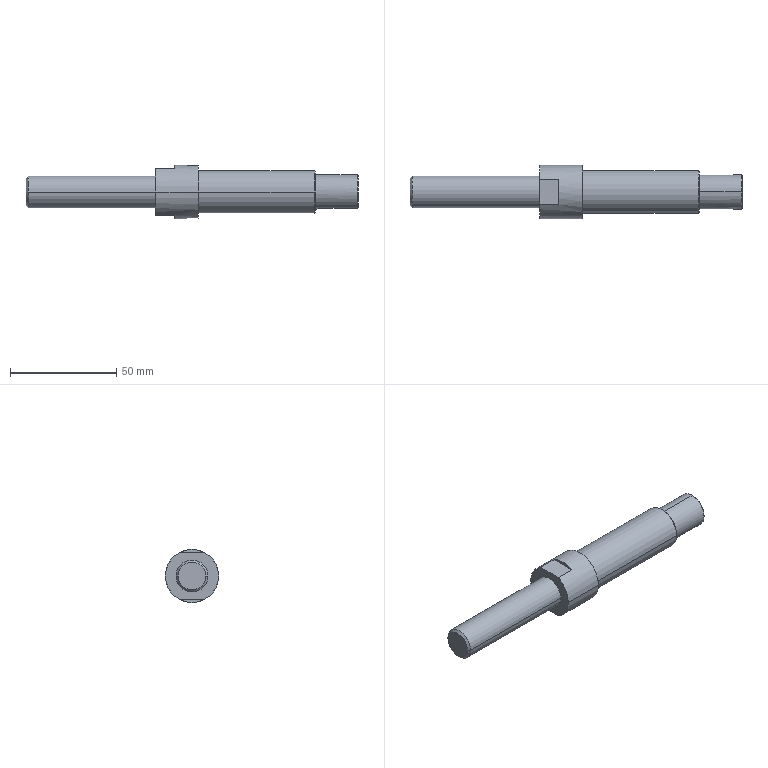Part | NX | 1 solid | 29 faces | box 156 x 25 x 25 mm | volume 41405 mm3 | plane 12 | cylinder 10 | cone 7 | commonest cylinder face diameters 5 x2 15 x2 16 x2 20 x2 25 x2
STEP:
#1=CARTESIAN_POINT('',(1862.,-10.,0.));
#2=VERTEX_POINT('',#1);
#3=CARTESIAN_POINT('',(1862.,10.,0.));
#4=VERTEX_POINT('',#3);
#5=CARTESIAN_POINT('',(1862.,0.,0.));
#6=DIRECTION('',(1.,0.,0.));
#7=DIRECTION('',(0.,1.,0.));
#8=AXIS2_PLACEMENT_3D('',#5,#6,#7);
#9=CIRCLE('',#8,10.);
#10=EDGE_CURVE('',#2,#4,#9,.T.);
#11=ORIENTED_EDGE('',*,*,#10,.T.);
#12=CARTESIAN_POINT('',(1916.5,10.,0.));
#13=VERTEX_POINT('',#12);
#14=CARTESIAN_POINT('',(1862.,10.,0.));
#15=DIRECTION('',(1.,0.,0.));
#16=VECTOR('',#15,1000.);
#17=LINE('',#14,#16);
#18=EDGE_CURVE('',#4,#13,#17,.T.);
#19=ORIENTED_EDGE('',*,*,#18,.T.);
#20=CARTESIAN_POINT('',(1916.5,-10.,0.));
#21=VERTEX_POINT('',#20);
#22=CARTESIAN_POINT('',(1916.5,0.,0.));
#23=DIRECTION('',(-1.,0.,0.));
#24=DIRECTION('',(0.,1.,0.));
#25=AXIS2_PLACEMENT_3D('',#22,#23,#24);
#26=CIRCLE('',#25,10.);
#27=EDGE_CURVE('',#13,#21,#26,.T.);
#28=ORIENTED_EDGE('',*,*,#27,.T.);
#29=CARTESIAN_POINT('',(1862.,-10.,0.));
#30=DIRECTION('',(1.,0.,0.));
#31=VECTOR('',#30,1000.);
#32=LINE('',#29,#31);
#33=EDGE_CURVE('',#2,#21,#32,.T.);
#34=ORIENTED_EDGE('',*,*,#33,.F.);
#35=EDGE_LOOP('',(#11,#19,#28,#34));
#36=FACE_BOUND('',#35,.T.);
#37=CARTESIAN_POINT('',(1862.,0.,0.));
#38=DIRECTION('',(1.,0.,0.));
#39=DIRECTION('',(0.,1.,0.));
#40=AXIS2_PLACEMENT_3D('',#37,#38,#39);
#41=CYLINDRICAL_SURFACE('',#40,10.);
#42=ADVANCED_FACE('',(#36),#41,.T.);
#43=CARTESIAN_POINT('',(1862.,12.5,0.));
#44=VERTEX_POINT('',#43);
#45=CARTESIAN_POINT('',(1862.,-12.5,0.));
#46=VERTEX_POINT('',#45);
#47=CARTESIAN_POINT('',(1862.,0.,0.));
#48=DIRECTION('',(-1.,0.,0.));
#49=DIRECTION('',(0.,1.,0.));
#50=AXIS2_PLACEMENT_3D('',#47,#48,#49);
#51=CIRCLE('',#50,12.5);
#52=EDGE_CURVE('',#44,#46,#51,.T.);
#53=ORIENTED_EDGE('',*,*,#52,.F.);
#54=CARTESIAN_POINT('',(1862.,0.,0.));
#55=DIRECTION('',(-1.,0.,0.));
#56=DIRECTION('',(0.,1.,0.));
#57=AXIS2_PLACEMENT_3D('',#54,#55,#56);
#58=CIRCLE('',#57,12.5);
#59=EDGE_CURVE('',#46,#44,#58,.T.);
#60=ORIENTED_EDGE('',*,*,#59,.F.);
#61=EDGE_LOOP('',(#53,#60));
#62=FACE_BOUND('',#61,.T.);
#63=ORIENTED_EDGE('',*,*,#10,.F.);
#64=CARTESIAN_POINT('',(1862.,0.,0.));
#65=DIRECTION('',(1.,0.,0.));
#66=DIRECTION('',(0.,1.,0.));
#67=AXIS2_PLACEMENT_3D('',#64,#65,#66);
#68=CIRCLE('',#67,10.);
#69=EDGE_CURVE('',#4,#2,#68,.T.);
#70=ORIENTED_EDGE('',*,*,#69,.F.);
#71=EDGE_LOOP('',(#63,#70));
#72=FACE_BOUND('',#71,.T.);
#73=CARTESIAN_POINT('',(1862.,-2.339,-2.068));
#74=DIRECTION('',(-1.,0.,0.));
#75=DIRECTION('',(0.,0.,1.));
#76=AXIS2_PLACEMENT_3D('',#73,#74,#75);
#77=PLANE('',#76);
#78=ADVANCED_FACE('',(#62,#72),#77,.F.);
#79=CARTESIAN_POINT('',(1842.,12.5,0.));
#80=VERTEX_POINT('',#79);
#81=CARTESIAN_POINT('',(1842.,5.937,-11.));
#82=VERTEX_POINT('',#81);
#83=CARTESIAN_POINT('',(1842.,0.,0.));
#84=DIRECTION('',(-1.,0.,0.));
#85=DIRECTION('',(0.,1.,0.));
#86=AXIS2_PLACEMENT_3D('',#83,#84,#85);
#87=CIRCLE('',#86,12.5);
#88=EDGE_CURVE('',#80,#82,#87,.T.);
#89=ORIENTED_EDGE('',*,*,#88,.T.);
#90=CARTESIAN_POINT('',(1842.,-5.937,-11.));
#91=VERTEX_POINT('',#90);
#92=CARTESIAN_POINT('',(1842.,3.345,-11.));
#93=DIRECTION('',(0.,1.,0.));
#94=VECTOR('',#93,1000.);
#95=LINE('',#92,#94);
#96=EDGE_CURVE('',#91,#82,#95,.T.);
#97=ORIENTED_EDGE('',*,*,#96,.F.);
#98=CARTESIAN_POINT('',(1842.,-12.5,0.));
#99=VERTEX_POINT('',#98);
#100=CARTESIAN_POINT('',(1842.,0.,0.));
#101=DIRECTION('',(-1.,0.,0.));
#102=DIRECTION('',(0.,1.,0.));
#103=AXIS2_PLACEMENT_3D('',#100,#101,#102);
#104=CIRCLE('',#103,12.5);
#105=EDGE_CURVE('',#91,#99,#104,.T.);
#106=ORIENTED_EDGE('',*,*,#105,.T.);
#107=CARTESIAN_POINT('',(1842.,-5.937,11.));
#108=VERTEX_POINT('',#107);
#109=CARTESIAN_POINT('',(1842.,0.,0.));
#110=DIRECTION('',(-1.,0.,0.));
#111=DIRECTION('',(0.,1.,0.));
#112=AXIS2_PLACEMENT_3D('',#109,#110,#111);
#113=CIRCLE('',#112,12.5);
#114=EDGE_CURVE('',#99,#108,#113,.T.);
#115=ORIENTED_EDGE('',*,*,#114,.T.);
#116=CARTESIAN_POINT('',(1842.,5.937,11.));
#117=VERTEX_POINT('',#116);
#118=CARTESIAN_POINT('',(1842.,3.345,11.));
#119=DIRECTION('',(0.,-1.,0.));
#120=VECTOR('',#119,1000.);
#121=LINE('',#118,#120);
#122=EDGE_CURVE('',#117,#108,#121,.T.);
#123=ORIENTED_EDGE('',*,*,#122,.F.);
#124=CARTESIAN_POINT('',(1842.,0.,0.));
#125=DIRECTION('',(-1.,0.,0.));
#126=DIRECTION('',(0.,1.,0.));
#127=AXIS2_PLACEMENT_3D('',#124,#125,#126);
#128=CIRCLE('',#127,12.5);
#129=EDGE_CURVE('',#117,#80,#128,.T.);
#130=ORIENTED_EDGE('',*,*,#129,.T.);
#131=EDGE_LOOP('',(#89,#97,#106,#115,#123,#130));
#132=FACE_BOUND('',#131,.T.);
#133=CARTESIAN_POINT('',(1842.,-7.5,0.));
#134=VERTEX_POINT('',#133);
#135=CARTESIAN_POINT('',(1842.,7.5,0.));
#136=VERTEX_POINT('',#135);
#137=CARTESIAN_POINT('',(1842.,0.,0.));
#138=DIRECTION('',(-1.,0.,0.));
#139=DIRECTION('',(0.,-1.,0.));
#140=AXIS2_PLACEMENT_3D('',#137,#138,#139);
#141=CIRCLE('',#140,7.5);
#142=EDGE_CURVE('',#134,#136,#141,.T.);
#143=ORIENTED_EDGE('',*,*,#142,.F.);
#144=CARTESIAN_POINT('',(1842.,0.,0.));
#145=DIRECTION('',(-1.,0.,0.));
#146=DIRECTION('',(0.,-1.,0.));
#147=AXIS2_PLACEMENT_3D('',#144,#145,#146);
#148=CIRCLE('',#147,7.5);
#149=EDGE_CURVE('',#136,#134,#148,.T.);
#150=ORIENTED_EDGE('',*,*,#149,.F.);
#151=EDGE_LOOP('',(#143,#150));
#152=FACE_BOUND('',#151,.T.);
#153=CARTESIAN_POINT('',(1842.,-2.339,-2.068));
#154=DIRECTION('',(-1.,0.,0.));
#155=DIRECTION('',(0.,0.,1.));
#156=AXIS2_PLACEMENT_3D('',#153,#154,#155);
#157=PLANE('',#156);
#158=ADVANCED_FACE('',(#132,#152),#157,.T.);
#159=ORIENTED_EDGE('',*,*,#52,.T.);
#160=CARTESIAN_POINT('',(1862.,-12.5,0.));
#161=DIRECTION('',(-1.,0.,0.));
#162=VECTOR('',#161,1000.);
#163=LINE('',#160,#162);
#164=EDGE_CURVE('',#99,#46,#163,.F.);
#165=ORIENTED_EDGE('',*,*,#164,.F.);
#166=ORIENTED_EDGE('',*,*,#105,.F.);
#167=CARTESIAN_POINT('',(1851.,-5.937,-11.));
#168=VERTEX_POINT('',#167);
#169=CARTESIAN_POINT('',(1862.,-5.937,-11.));
#170=DIRECTION('',(-1.,0.,0.));
#171=VECTOR('',#170,1000.);
#172=LINE('',#169,#171);
#173=EDGE_CURVE('',#91,#168,#172,.F.);
#174=ORIENTED_EDGE('',*,*,#173,.T.);
#175=CARTESIAN_POINT('',(1851.,5.937,-11.));
#176=VERTEX_POINT('',#175);
#177=CARTESIAN_POINT('',(1851.,0.,0.));
#178=DIRECTION('',(-1.,0.,0.));
#179=DIRECTION('',(0.,1.,0.));
#180=AXIS2_PLACEMENT_3D('',#177,#178,#179);
#181=CIRCLE('',#180,12.5);
#182=EDGE_CURVE('',#176,#168,#181,.T.);
#183=ORIENTED_EDGE('',*,*,#182,.F.);
#184=CARTESIAN_POINT('',(1862.,5.937,-11.));
#185=DIRECTION('',(-1.,0.,0.));
#186=VECTOR('',#185,1000.);
#187=LINE('',#184,#186);
#188=EDGE_CURVE('',#82,#176,#187,.F.);
#189=ORIENTED_EDGE('',*,*,#188,.F.);
#190=ORIENTED_EDGE('',*,*,#88,.F.);
#191=CARTESIAN_POINT('',(1862.,12.5,0.));
#192=DIRECTION('',(-1.,0.,0.));
#193=VECTOR('',#192,1000.);
#194=LINE('',#191,#193);
#195=EDGE_CURVE('',#80,#44,#194,.F.);
#196=ORIENTED_EDGE('',*,*,#195,.T.);
#197=EDGE_LOOP('',(#159,#165,#166,#174,#183,#189,#190,#196));
#198=FACE_BOUND('',#197,.T.);
#199=CARTESIAN_POINT('',(1862.,0.,0.));
#200=DIRECTION('',(-1.,0.,0.));
#201=DIRECTION('',(0.,1.,0.));
#202=AXIS2_PLACEMENT_3D('',#199,#200,#201);
#203=CYLINDRICAL_SURFACE('',#202,12.5);
#204=ADVANCED_FACE('',(#198),#203,.T.);
#205=CARTESIAN_POINT('',(1920.,-2.5,-7.599));
#206=VERTEX_POINT('',#205);
#207=CARTESIAN_POINT('',(1920.,-2.5,-5.3));
#208=VERTEX_POINT('',#207);
#209=CARTESIAN_POINT('',(1920.,-2.5,-10.5));
#210=DIRECTION('',(0.,0.,1.));
#211=VECTOR('',#210,1000.);
#212=LINE('',#209,#211);
#213=EDGE_CURVE('',#206,#208,#212,.T.);
#214=ORIENTED_EDGE('',*,*,#213,.T.);
#215=CARTESIAN_POINT('',(1937.,-2.5,-5.3));
#216=VERTEX_POINT('',#215);
#217=CARTESIAN_POINT('',(1920.,-2.5,-5.3));
#218=DIRECTION('',(1.,0.,0.));
#219=VECTOR('',#218,1000.);
#220=LINE('',#217,#219);
#221=EDGE_CURVE('',#208,#216,#220,.T.);
#222=ORIENTED_EDGE('',*,*,#221,.T.);
#223=CARTESIAN_POINT('',(1937.,-2.5,-7.283));
#224=VERTEX_POINT('',#223);
#225=CARTESIAN_POINT('',(1937.,-2.5,-12.278));
#226=DIRECTION('',(0.,0.,-1.));
#227=VECTOR('',#226,1000.);
#228=LINE('',#225,#227);
#229=EDGE_CURVE('',#216,#224,#228,.T.);
#230=ORIENTED_EDGE('',*,*,#229,.T.);
#231=CARTESIAN_POINT('',(1936.7,-2.5,-7.599));
#232=VERTEX_POINT('',#231);
#233=CARTESIAN_POINT('',(1937.,-2.5,-7.283));
#234=CARTESIAN_POINT('',(1936.988,-2.5,-7.296));
#235=CARTESIAN_POINT('',(1936.975,-2.5,-7.309));
#236=CARTESIAN_POINT('',(1936.963,-2.5,-7.322));
#237=CARTESIAN_POINT('',(1936.95,-2.5,-7.336));
#238=CARTESIAN_POINT('',(1936.938,-2.5,-7.349));
#239=CARTESIAN_POINT('',(1936.925,-2.5,-7.362));
#240=CARTESIAN_POINT('',(1936.9,-2.5,-7.388));
#241=CARTESIAN_POINT('',(1936.875,-2.5,-7.415));
#242=CARTESIAN_POINT('',(1936.85,-2.5,-7.441));
#243=CARTESIAN_POINT('',(1936.825,-2.5,-7.468));
#244=CARTESIAN_POINT('',(1936.8,-2.5,-7.494));
#245=CARTESIAN_POINT('',(1936.775,-2.5,-7.52));
#246=CARTESIAN_POINT('',(1936.75,-2.5,-7.547));
#247=CARTESIAN_POINT('',(1936.725,-2.5,-7.573));
#248=CARTESIAN_POINT('',(1936.7,-2.5,-7.599));
#249=B_SPLINE_CURVE_WITH_KNOTS('',3,(#233,#234,#235,#236,#237,#238,#239,#240,#241,#242,#243,#244,#245,#246,#247,#248),.UNSPECIFIED.,.F.,.F.,(4,3,3,3,3,4),(0.,0.05451,0.109,0.218,0.3271,0.4361),.UNSPECIFIED.);
#250=EDGE_CURVE('',#224,#232,#249,.T.);
#251=ORIENTED_EDGE('',*,*,#250,.T.);
#252=CARTESIAN_POINT('',(1937.,-2.5,-7.599));
#253=DIRECTION('',(1.,0.,0.));
#254=VECTOR('',#253,1000.);
#255=LINE('',#252,#254);
#256=EDGE_CURVE('',#206,#232,#255,.T.);
#257=ORIENTED_EDGE('',*,*,#256,.F.);
#258=EDGE_LOOP('',(#214,#222,#230,#251,#257));
#259=FACE_BOUND('',#258,.T.);
#260=CARTESIAN_POINT('',(1939.409,-2.5,-10.5));
#261=DIRECTION('',(0.,-1.,0.));
#262=DIRECTION('',(0.,0.,-1.));
#263=AXIS2_PLACEMENT_3D('',#260,#261,#262);
#264=PLANE('',#263);
#265=ADVANCED_FACE('',(#259),#264,.F.);
#266=CARTESIAN_POINT('',(1937.,7.7,0.));
#267=VERTEX_POINT('',#266);
#268=CARTESIAN_POINT('',(1936.7,8.,0.));
#269=VERTEX_POINT('',#268);
#270=CARTESIAN_POINT('',(1937.,7.7,0.));
#271=DIRECTION('',(-0.7071,0.7071,0.));
#272=VECTOR('',#271,1000.);
#273=LINE('',#270,#272);
#274=EDGE_CURVE('',#267,#269,#273,.T.);
#275=ORIENTED_EDGE('',*,*,#274,.F.);
#276=CARTESIAN_POINT('',(1937.,2.5,-7.283));
#277=VERTEX_POINT('',#276);
#278=CARTESIAN_POINT('',(1937.,0.,0.));
#279=DIRECTION('',(1.,0.,0.));
#280=DIRECTION('',(0.,1.,0.));
#281=AXIS2_PLACEMENT_3D('',#278,#279,#280);
#282=CIRCLE('',#281,7.7);
#283=EDGE_CURVE('',#277,#267,#282,.T.);
#284=ORIENTED_EDGE('',*,*,#283,.F.);
#285=CARTESIAN_POINT('',(1936.7,2.5,-7.599));
#286=VERTEX_POINT('',#285);
#287=CARTESIAN_POINT('',(1936.7,2.5,-7.599));
#288=CARTESIAN_POINT('',(1936.725,2.5,-7.573));
#289=CARTESIAN_POINT('',(1936.75,2.5,-7.547));
#290=CARTESIAN_POINT('',(1936.775,2.5,-7.52));
#291=CARTESIAN_POINT('',(1936.8,2.5,-7.494));
#292=CARTESIAN_POINT('',(1936.825,2.5,-7.468));
#293=CARTESIAN_POINT('',(1936.85,2.5,-7.441));
#294=CARTESIAN_POINT('',(1936.875,2.5,-7.415));
#295=CARTESIAN_POINT('',(1936.9,2.5,-7.388));
#296=CARTESIAN_POINT('',(1936.925,2.5,-7.362));
#297=CARTESIAN_POINT('',(1936.95,2.5,-7.336));
#298=CARTESIAN_POINT('',(1936.975,2.5,-7.309));
#299=CARTESIAN_POINT('',(1937.,2.5,-7.283));
#300=B_SPLINE_CURVE_WITH_KNOTS('',3,(#287,#288,#289,#290,#291,#292,#293,#294,#295,#296,#297,#298,#299),.UNSPECIFIED.,.F.,.F.,(4,3,3,3,4),(0.,0.109,0.218,0.3271,0.4361),.UNSPECIFIED.);
#301=EDGE_CURVE('',#286,#277,#300,.T.);
#302=ORIENTED_EDGE('',*,*,#301,.F.);
#303=CARTESIAN_POINT('',(1936.7,0.,0.));
#304=DIRECTION('',(-1.,0.,0.));
#305=DIRECTION('',(0.,1.,0.));
#306=AXIS2_PLACEMENT_3D('',#303,#304,#305);
#307=CIRCLE('',#306,8.);
#308=EDGE_CURVE('',#269,#286,#307,.T.);
#309=ORIENTED_EDGE('',*,*,#308,.F.);
#310=EDGE_LOOP('',(#275,#284,#302,#309));
#311=FACE_BOUND('',#310,.T.);
#312=CARTESIAN_POINT('',(1937.,0.,0.));
#313=DIRECTION('',(-1.,0.,0.));
#314=DIRECTION('',(0.,1.,0.));
#315=AXIS2_PLACEMENT_3D('',#312,#313,#314);
#316=CONICAL_SURFACE('',#315,7.7,0.7854);
#317=ADVANCED_FACE('',(#311),#316,.T.);
#318=ORIENTED_EDGE('',*,*,#142,.T.);
#319=CARTESIAN_POINT('',(1782.,7.5,0.));
#320=VERTEX_POINT('',#319);
#321=CARTESIAN_POINT('',(1847.,7.5,0.));
#322=DIRECTION('',(-1.,0.,0.));
#323=VECTOR('',#322,1000.);
#324=LINE('',#321,#323);
#325=EDGE_CURVE('',#136,#320,#324,.T.);
#326=ORIENTED_EDGE('',*,*,#325,.T.);
#327=CARTESIAN_POINT('',(1782.,-7.5,0.));
#328=VERTEX_POINT('',#327);
#329=CARTESIAN_POINT('',(1782.,0.,0.));
#330=DIRECTION('',(-1.,0.,0.));
#331=DIRECTION('',(0.,-1.,0.));
#332=AXIS2_PLACEMENT_3D('',#329,#330,#331);
#333=CIRCLE('',#332,7.5);
#334=EDGE_CURVE('',#328,#320,#333,.T.);
#335=ORIENTED_EDGE('',*,*,#334,.F.);
#336=CARTESIAN_POINT('',(1847.,-7.5,0.));
#337=DIRECTION('',(-1.,0.,0.));
#338=VECTOR('',#337,1000.);
#339=LINE('',#336,#338);
#340=EDGE_CURVE('',#134,#328,#339,.T.);
#341=ORIENTED_EDGE('',*,*,#340,.F.);
#342=EDGE_LOOP('',(#318,#326,#335,#341));
#343=FACE_BOUND('',#342,.T.);
#344=CARTESIAN_POINT('',(1847.,0.,0.));
#345=DIRECTION('',(-1.,0.,0.));
#346=DIRECTION('',(0.,-1.,0.));
#347=AXIS2_PLACEMENT_3D('',#344,#345,#346);
#348=CYLINDRICAL_SURFACE('',#347,7.5);
#349=ADVANCED_FACE('',(#343),#348,.T.);
#350=CARTESIAN_POINT('',(1781.,-6.5,0.));
#351=VERTEX_POINT('',#350);
#352=CARTESIAN_POINT('',(1781.,6.5,0.));
#353=VERTEX_POINT('',#352);
#354=CARTESIAN_POINT('',(1781.,0.,0.));
#355=DIRECTION('',(-1.,0.,0.));
#356=DIRECTION('',(0.,-1.,0.));
#357=AXIS2_PLACEMENT_3D('',#354,#355,#356);
#358=CIRCLE('',#357,6.5);
#359=EDGE_CURVE('',#351,#353,#358,.T.);
#360=ORIENTED_EDGE('',*,*,#359,.T.);
#361=CARTESIAN_POINT('',(1781.,0.,0.));
#362=DIRECTION('',(-1.,0.,0.));
#363=DIRECTION('',(0.,-1.,0.));
#364=AXIS2_PLACEMENT_3D('',#361,#362,#363);
#365=CIRCLE('',#364,6.5);
#366=EDGE_CURVE('',#353,#351,#365,.T.);
#367=ORIENTED_EDGE('',*,*,#366,.T.);
#368=EDGE_LOOP('',(#360,#367));
#369=FACE_BOUND('',#368,.T.);
#370=CARTESIAN_POINT('',(1781.,-3.365,-3.262));
#371=DIRECTION('',(-1.,0.,0.));
#372=DIRECTION('',(0.,0.,1.));
#373=AXIS2_PLACEMENT_3D('',#370,#371,#372);
#374=PLANE('',#373);
#375=ADVANCED_FACE('',(#369),#374,.T.);
#376=ORIENTED_EDGE('',*,*,#182,.T.);
#377=CARTESIAN_POINT('',(1851.,12.771,-11.));
#378=DIRECTION('',(0.,-1.,0.));
#379=VECTOR('',#378,1000.);
#380=LINE('',#377,#379);
#381=EDGE_CURVE('',#176,#168,#380,.T.);
#382=ORIENTED_EDGE('',*,*,#381,.F.);
#383=EDGE_LOOP('',(#376,#382));
#384=FACE_BOUND('',#383,.T.);
#385=CARTESIAN_POINT('',(1851.,0.0706,-2.347));
#386=DIRECTION('',(-1.,0.,0.));
#387=DIRECTION('',(0.,0.,1.));
#388=AXIS2_PLACEMENT_3D('',#385,#386,#387);
#389=PLANE('',#388);
#390=ADVANCED_FACE('',(#384),#389,.T.);
#391=ORIENTED_EDGE('',*,*,#173,.F.);
#392=ORIENTED_EDGE('',*,*,#96,.T.);
#393=ORIENTED_EDGE('',*,*,#188,.T.);
#394=ORIENTED_EDGE('',*,*,#381,.T.);
#395=EDGE_LOOP('',(#391,#392,#393,#394));
#396=FACE_BOUND('',#395,.T.);
#397=CARTESIAN_POINT('',(1822.,-14.229,-11.));
#398=DIRECTION('',(0.,0.,1.));
#399=DIRECTION('',(1.,0.,0.));
#400=AXIS2_PLACEMENT_3D('',#397,#398,#399);
#401=PLANE('',#400);
#402=ADVANCED_FACE('',(#396),#401,.F.);
#403=CARTESIAN_POINT('',(1851.,-5.937,11.));
#404=VERTEX_POINT('',#403);
#405=CARTESIAN_POINT('',(1851.,5.937,11.));
#406=VERTEX_POINT('',#405);
#407=CARTESIAN_POINT('',(1851.,0.,0.));
#408=DIRECTION('',(-1.,0.,0.));
#409=DIRECTION('',(0.,1.,0.));
#410=AXIS2_PLACEMENT_3D('',#407,#408,#409);
#411=CIRCLE('',#410,12.5);
#412=EDGE_CURVE('',#404,#406,#411,.T.);
#413=ORIENTED_EDGE('',*,*,#412,.T.);
#414=CARTESIAN_POINT('',(1851.,12.771,11.));
#415=DIRECTION('',(0.,-1.,0.));
#416=VECTOR('',#415,1000.);
#417=LINE('',#414,#416);
#418=EDGE_CURVE('',#406,#404,#417,.T.);
#419=ORIENTED_EDGE('',*,*,#418,.T.);
#420=EDGE_LOOP('',(#413,#419));
#421=FACE_BOUND('',#420,.T.);
#422=CARTESIAN_POINT('',(1851.,0.0706,-2.347));
#423=DIRECTION('',(-1.,0.,0.));
#424=DIRECTION('',(0.,0.,1.));
#425=AXIS2_PLACEMENT_3D('',#422,#423,#424);
#426=PLANE('',#425);
#427=ADVANCED_FACE('',(#421),#426,.T.);
#428=CARTESIAN_POINT('',(1862.,5.937,11.));
#429=DIRECTION('',(-1.,0.,0.));
#430=VECTOR('',#429,1000.);
#431=LINE('',#428,#430);
#432=EDGE_CURVE('',#406,#117,#431,.T.);
#433=ORIENTED_EDGE('',*,*,#432,.T.);
#434=ORIENTED_EDGE('',*,*,#122,.T.);
#435=CARTESIAN_POINT('',(1862.,-5.937,11.));
#436=DIRECTION('',(-1.,0.,0.));
#437=VECTOR('',#436,1000.);
#438=LINE('',#435,#437);
#439=EDGE_CURVE('',#404,#108,#438,.T.);
#440=ORIENTED_EDGE('',*,*,#439,.F.);
#441=ORIENTED_EDGE('',*,*,#418,.F.);
#442=EDGE_LOOP('',(#433,#434,#440,#441));
#443=FACE_BOUND('',#442,.T.);
#444=CARTESIAN_POINT('',(1822.,12.771,11.));
#445=DIRECTION('',(0.,0.,-1.));
#446=DIRECTION('',(0.,-1.,0.));
#447=AXIS2_PLACEMENT_3D('',#444,#445,#446);
#448=PLANE('',#447);
#449=ADVANCED_FACE('',(#443),#448,.F.);
#450=ORIENTED_EDGE('',*,*,#359,.F.);
#451=CARTESIAN_POINT('',(1781.,-6.5,0.));
#452=DIRECTION('',(0.7071,-0.7071,0.));
#453=VECTOR('',#452,1000.);
#454=LINE('',#451,#453);
#455=EDGE_CURVE('',#328,#351,#454,.F.);
#456=ORIENTED_EDGE('',*,*,#455,.F.);
#457=ORIENTED_EDGE('',*,*,#334,.T.);
#458=CARTESIAN_POINT('',(1781.,6.5,0.));
#459=DIRECTION('',(0.7071,0.7071,0.));
#460=VECTOR('',#459,1000.);
#461=LINE('',#458,#460);
#462=EDGE_CURVE('',#320,#353,#461,.F.);
#463=ORIENTED_EDGE('',*,*,#462,.T.);
#464=EDGE_LOOP('',(#450,#456,#457,#463));
#465=FACE_BOUND('',#464,.T.);
#466=CARTESIAN_POINT('',(1781.,0.,0.));
#467=DIRECTION('',(1.,0.,0.));
#468=DIRECTION('',(0.,-1.,0.));
#469=AXIS2_PLACEMENT_3D('',#466,#467,#468);
#470=CONICAL_SURFACE('',#469,6.5,0.7854);
#471=ADVANCED_FACE('',(#465),#470,.T.);
#472=ORIENTED_EDGE('',*,*,#283,.T.);
#473=CARTESIAN_POINT('',(1937.,-7.7,0.));
#474=VERTEX_POINT('',#473);
#475=CARTESIAN_POINT('',(1937.,0.,0.));
#476=DIRECTION('',(1.,0.,0.));
#477=DIRECTION('',(0.,1.,0.));
#478=AXIS2_PLACEMENT_3D('',#475,#476,#477);
#479=CIRCLE('',#478,7.7);
#480=EDGE_CURVE('',#267,#474,#479,.T.);
#481=ORIENTED_EDGE('',*,*,#480,.T.);
#482=CARTESIAN_POINT('',(1937.,0.,0.));
#483=DIRECTION('',(1.,0.,0.));
#484=DIRECTION('',(0.,1.,0.));
#485=AXIS2_PLACEMENT_3D('',#482,#483,#484);
#486=CIRCLE('',#485,7.7);
#487=EDGE_CURVE('',#474,#224,#486,.T.);
#488=ORIENTED_EDGE('',*,*,#487,.T.);
#489=ORIENTED_EDGE('',*,*,#229,.F.);
#490=CARTESIAN_POINT('',(1937.,2.5,-5.3));
#491=VERTEX_POINT('',#490);
#492=CARTESIAN_POINT('',(1937.,3.345,-5.3));
#493=DIRECTION('',(0.,-1.,0.));
#494=VECTOR('',#493,1000.);
#495=LINE('',#492,#494);
#496=EDGE_CURVE('',#491,#216,#495,.T.);
#497=ORIENTED_EDGE('',*,*,#496,.F.);
#498=CARTESIAN_POINT('',(1937.,2.5,-12.278));
#499=DIRECTION('',(0.,0.,1.));
#500=VECTOR('',#499,1000.);
#501=LINE('',#498,#500);
#502=EDGE_CURVE('',#277,#491,#501,.T.);
#503=ORIENTED_EDGE('',*,*,#502,.F.);
#504=EDGE_LOOP('',(#472,#481,#488,#489,#497,#503));
#505=FACE_BOUND('',#504,.T.);
#506=CARTESIAN_POINT('',(1937.,-0.2257,-0.6793));
#507=DIRECTION('',(1.,0.,0.));
#508=DIRECTION('',(0.,1.,0.));
#509=AXIS2_PLACEMENT_3D('',#506,#507,#508);
#510=PLANE('',#509);
#511=ADVANCED_FACE('',(#505),#510,.T.);
#512=CARTESIAN_POINT('',(1917.5,0.,-8.));
#513=VERTEX_POINT('',#512);
#514=CARTESIAN_POINT('',(1917.5,0.,-5.3));
#515=VERTEX_POINT('',#514);
#516=CARTESIAN_POINT('',(1917.5,0.,-10.5));
#517=DIRECTION('',(0.,0.,1.));
#518=VECTOR('',#517,1000.);
#519=LINE('',#516,#518);
#520=EDGE_CURVE('',#513,#515,#519,.T.);
#521=ORIENTED_EDGE('',*,*,#520,.F.);
#522=CARTESIAN_POINT('',(1920.,2.5,-7.599));
#523=VERTEX_POINT('',#522);
#524=CARTESIAN_POINT('',(1920.,2.5,-7.599));
#525=CARTESIAN_POINT('',(1919.959,2.5,-7.599));
#526=CARTESIAN_POINT('',(1919.918,2.499,-7.6));
#527=CARTESIAN_POINT('',(1919.877,2.497,-7.6));
#528=CARTESIAN_POINT('',(1919.856,2.496,-7.601));
#529=CARTESIAN_POINT('',(1919.836,2.495,-7.601));
#530=CARTESIAN_POINT('',(1919.815,2.493,-7.602));
#531=CARTESIAN_POINT('',(1919.795,2.492,-7.602));
#532=CARTESIAN_POINT('',(1919.774,2.49,-7.603));
#533=CARTESIAN_POINT('',(1919.754,2.488,-7.603));
#534=CARTESIAN_POINT('',(1919.713,2.484,-7.605));
#535=CARTESIAN_POINT('',(1919.672,2.479,-7.606));
#536=CARTESIAN_POINT('',(1919.632,2.473,-7.608));
#537=CARTESIAN_POINT('',(1919.591,2.467,-7.61));
#538=CARTESIAN_POINT('',(1919.55,2.46,-7.613));
#539=CARTESIAN_POINT('',(1919.51,2.451,-7.615));
#540=CARTESIAN_POINT('',(1919.47,2.443,-7.618));
#541=CARTESIAN_POINT('',(1919.429,2.434,-7.621));
#542=CARTESIAN_POINT('',(1919.389,2.424,-7.624));
#543=CARTESIAN_POINT('',(1919.349,2.414,-7.627));
#544=CARTESIAN_POINT('',(1919.31,2.403,-7.631));
#545=CARTESIAN_POINT('',(1919.27,2.391,-7.634));
#546=CARTESIAN_POINT('',(1919.231,2.379,-7.638));
#547=CARTESIAN_POINT('',(1919.192,2.366,-7.642));
#548=CARTESIAN_POINT('',(1919.153,2.352,-7.646));
#549=CARTESIAN_POINT('',(1919.114,2.338,-7.651));
#550=CARTESIAN_POINT('',(1919.076,2.323,-7.655));
#551=CARTESIAN_POINT('',(1919.038,2.308,-7.66));
#552=CARTESIAN_POINT('',(1919.001,2.292,-7.665));
#553=CARTESIAN_POINT('',(1918.963,2.275,-7.67));
#554=CARTESIAN_POINT('',(1918.927,2.258,-7.675));
#555=CARTESIAN_POINT('',(1918.89,2.24,-7.68));
#556=CARTESIAN_POINT('',(1918.854,2.222,-7.685));
#557=CARTESIAN_POINT('',(1918.818,2.203,-7.691));
#558=CARTESIAN_POINT('',(1918.782,2.184,-7.696));
#559=CARTESIAN_POINT('',(1918.746,2.163,-7.702));
#560=CARTESIAN_POINT('',(1918.711,2.142,-7.708));
#561=CARTESIAN_POINT('',(1918.677,2.121,-7.714));
#562=CARTESIAN_POINT('',(1918.642,2.099,-7.72));
#563=CARTESIAN_POINT('',(1918.608,2.077,-7.726));
#564=CARTESIAN_POINT('',(1918.574,2.054,-7.732));
#565=CARTESIAN_POINT('',(1918.541,2.03,-7.738));
#566=CARTESIAN_POINT('',(1918.508,2.006,-7.744));
#567=CARTESIAN_POINT('',(1918.475,1.982,-7.751));
#568=CARTESIAN_POINT('',(1918.443,1.956,-7.757));
#569=CARTESIAN_POINT('',(1918.411,1.93,-7.764));
#570=CARTESIAN_POINT('',(1918.38,1.904,-7.77));
#571=CARTESIAN_POINT('',(1918.349,1.878,-7.777));
#572=CARTESIAN_POINT('',(1918.319,1.85,-7.783));
#573=CARTESIAN_POINT('',(1918.289,1.823,-7.79));
#574=CARTESIAN_POINT('',(1918.259,1.795,-7.796));
#575=CARTESIAN_POINT('',(1918.23,1.766,-7.803));
#576=CARTESIAN_POINT('',(1918.202,1.737,-7.809));
#577=CARTESIAN_POINT('',(1918.174,1.708,-7.816));
#578=CARTESIAN_POINT('',(1918.147,1.678,-7.822));
#579=CARTESIAN_POINT('',(1918.133,1.663,-7.825));
#580=CARTESIAN_POINT('',(1918.12,1.647,-7.829));
#581=CARTESIAN_POINT('',(1918.106,1.632,-7.832));
#582=CARTESIAN_POINT('',(1918.093,1.617,-7.835));
#583=CARTESIAN_POINT('',(1918.08,1.601,-7.838));
#584=CARTESIAN_POINT('',(1918.067,1.586,-7.841));
#585=CARTESIAN_POINT('',(1918.041,1.554,-7.848));
#586=CARTESIAN_POINT('',(1918.016,1.522,-7.854));
#587=CARTESIAN_POINT('',(1917.992,1.489,-7.86));
#588=CARTESIAN_POINT('',(1917.968,1.457,-7.866));
#589=CARTESIAN_POINT('',(1917.944,1.423,-7.872));
#590=CARTESIAN_POINT('',(1917.922,1.389,-7.878));
#591=CARTESIAN_POINT('',(1917.899,1.355,-7.884));
#592=CARTESIAN_POINT('',(1917.877,1.321,-7.89));
#593=CARTESIAN_POINT('',(1917.856,1.286,-7.896));
#594=CARTESIAN_POINT('',(1917.835,1.251,-7.902));
#595=CARTESIAN_POINT('',(1917.815,1.215,-7.907));
#596=CARTESIAN_POINT('',(1917.795,1.179,-7.913));
#597=CARTESIAN_POINT('',(1917.776,1.143,-7.918));
#598=CARTESIAN_POINT('',(1917.758,1.106,-7.923));
#599=CARTESIAN_POINT('',(1917.74,1.069,-7.928));
#600=CARTESIAN_POINT('',(1917.723,1.032,-7.933));
#601=CARTESIAN_POINT('',(1917.706,0.9945,-7.938));
#602=CARTESIAN_POINT('',(1917.69,0.9567,-7.943));
#603=CARTESIAN_POINT('',(1917.675,0.9189,-7.947));
#604=CARTESIAN_POINT('',(1917.66,0.8808,-7.951));
#605=CARTESIAN_POINT('',(1917.646,0.8424,-7.956));
#606=CARTESIAN_POINT('',(1917.632,0.8039,-7.96));
#607=CARTESIAN_POINT('',(1917.62,0.7652,-7.963));
#608=CARTESIAN_POINT('',(1917.608,0.7261,-7.967));
#609=CARTESIAN_POINT('',(1917.596,0.687,-7.971));
#610=CARTESIAN_POINT('',(1917.585,0.6476,-7.974));
#611=CARTESIAN_POINT('',(1917.575,0.6079,-7.977));
#612=CARTESIAN_POINT('',(1917.565,0.5682,-7.98));
#613=CARTESIAN_POINT('',(1917.556,0.5283,-7.983));
#614=CARTESIAN_POINT('',(1917.548,0.4882,-7.985));
#615=CARTESIAN_POINT('',(1917.54,0.4481,-7.988));
#616=CARTESIAN_POINT('',(1917.533,0.4078,-7.99));
#617=CARTESIAN_POINT('',(1917.527,0.3673,-7.992));
#618=CARTESIAN_POINT('',(1917.521,0.3268,-7.993));
#619=CARTESIAN_POINT('',(1917.516,0.2861,-7.995));
#620=CARTESIAN_POINT('',(1917.512,0.2454,-7.996));
#621=CARTESIAN_POINT('',(1917.508,0.2046,-7.997));
#622=CARTESIAN_POINT('',(1917.505,0.1638,-7.998));
#623=CARTESIAN_POINT('',(1917.503,0.1228,-7.999));
#624=CARTESIAN_POINT('',(1917.501,0.08194,-8.));
#625=CARTESIAN_POINT('',(1917.5,0.04096,-8.));
#626=CARTESIAN_POINT('',(1917.5,0.,-8.));
#627=B_SPLINE_CURVE_WITH_KNOTS('',3,(#524,#525,#526,#527,#528,#529,#530,#531,#532,#533,#534,#535,#536,#537,#538,#539,#540,#541,#542,#543,#544,#545,#546,#547,#548,#549,#550,#551,#552,#553,#554,#555,#556,#557,#558,#559,#560,#561,#562,#563,#564,#565,#566,#567,#568,#569,#570,#571,#572,#573,#574,#575,#576,#577,#578,#579,#580,#581,#582,#583,#584,#585,#586,#587,#588,#589,#590,#591,#592,#593,#594,#595,#596,#597,#598,#599,#600,#601,#602,#603,#604,#605,#606,#607,#608,#609,#610,#611,#612,#613,#614,#615,#616,#617,#618,#619,#620,#621,#622,#623,#624,#625,#626),.UNSPECIFIED.,.F.,.F.,(4,3,3,3,3,3,3,3,3,3,3,3,3,3,3,3,3,3,3,3,3,3,3,3,3,3,3,3,3,3,3,3,3,3,4),(0.,0.1234,0.1849,0.2464,0.3698,0.4936,0.6176,0.7417,0.8657,0.9894,1.113,1.236,1.359,1.483,1.607,1.731,1.855,1.979,2.102,2.164,2.225,2.349,2.473,2.597,2.721,2.845,2.968,3.091,3.214,3.337,3.46,3.583,3.706,3.829,3.952),.UNSPECIFIED.);
#628=EDGE_CURVE('',#523,#513,#627,.T.);
#629=ORIENTED_EDGE('',*,*,#628,.F.);
#630=CARTESIAN_POINT('',(1920.,2.5,-5.3));
#631=VERTEX_POINT('',#630);
#632=CARTESIAN_POINT('',(1920.,2.5,-10.5));
#633=DIRECTION('',(0.,0.,1.));
#634=VECTOR('',#633,1000.);
#635=LINE('',#632,#634);
#636=EDGE_CURVE('',#523,#631,#635,.T.);
#637=ORIENTED_EDGE('',*,*,#636,.T.);
#638=CARTESIAN_POINT('',(1920.,0.,-5.3));
#639=DIRECTION('',(0.,0.,1.));
#640=DIRECTION('',(-1.,0.,0.));
#641=AXIS2_PLACEMENT_3D('',#638,#639,#640);
#642=CIRCLE('',#641,2.5);
#643=EDGE_CURVE('',#631,#515,#642,.T.);
#644=ORIENTED_EDGE('',*,*,#643,.T.);
#645=EDGE_LOOP('',(#521,#629,#637,#644));
#646=FACE_BOUND('',#645,.T.);
#647=CARTESIAN_POINT('',(1920.,0.,-10.5));
#648=DIRECTION('',(0.,0.,1.));
#649=DIRECTION('',(-1.,0.,0.));
#650=AXIS2_PLACEMENT_3D('',#647,#648,#649);
#651=CYLINDRICAL_SURFACE('',#650,2.5);
#652=ADVANCED_FACE('',(#646),#651,.F.);
#653=ORIENTED_EDGE('',*,*,#496,.T.);
#654=ORIENTED_EDGE('',*,*,#221,.F.);
#655=CARTESIAN_POINT('',(1920.,0.,-5.3));
#656=DIRECTION('',(0.,0.,1.));
#657=DIRECTION('',(-1.,0.,0.));
#658=AXIS2_PLACEMENT_3D('',#655,#656,#657);
#659=CIRCLE('',#658,2.5);
#660=EDGE_CURVE('',#515,#208,#659,.T.);
#661=ORIENTED_EDGE('',*,*,#660,.F.);
#662=ORIENTED_EDGE('',*,*,#643,.F.);
#663=CARTESIAN_POINT('',(1920.,2.5,-5.3));
#664=DIRECTION('',(1.,0.,0.));
#665=VECTOR('',#664,1000.);
#666=LINE('',#663,#665);
#667=EDGE_CURVE('',#631,#491,#666,.T.);
#668=ORIENTED_EDGE('',*,*,#667,.T.);
#669=EDGE_LOOP('',(#653,#654,#661,#662,#668));
#670=FACE_BOUND('',#669,.T.);
#671=CARTESIAN_POINT('',(1934.143,0.963,-5.3));
#672=DIRECTION('',(0.,0.,1.));
#673=DIRECTION('',(1.,0.,0.));
#674=AXIS2_PLACEMENT_3D('',#671,#672,#673);
#675=PLANE('',#674);
#676=ADVANCED_FACE('',(#670),#675,.F.);
#677=CARTESIAN_POINT('',(1937.,2.5,-7.599));
#678=DIRECTION('',(1.,0.,0.));
#679=VECTOR('',#678,1000.);
#680=LINE('',#677,#679);
#681=EDGE_CURVE('',#523,#286,#680,.T.);
#682=ORIENTED_EDGE('',*,*,#681,.T.);
#683=ORIENTED_EDGE('',*,*,#301,.T.);
#684=ORIENTED_EDGE('',*,*,#502,.T.);
#685=ORIENTED_EDGE('',*,*,#667,.F.);
#686=ORIENTED_EDGE('',*,*,#636,.F.);
#687=EDGE_LOOP('',(#682,#683,#684,#685,#686));
#688=FACE_BOUND('',#687,.T.);
#689=CARTESIAN_POINT('',(1920.,2.5,-10.5));
#690=DIRECTION('',(0.,1.,0.));
#691=DIRECTION('',(1.,0.,0.));
#692=AXIS2_PLACEMENT_3D('',#689,#690,#691);
#693=PLANE('',#692);
#694=ADVANCED_FACE('',(#688),#693,.F.);
#695=CARTESIAN_POINT('',(1917.,9.5,0.));
#696=VERTEX_POINT('',#695);
#697=CARTESIAN_POINT('',(1917.,-9.5,0.));
#698=VERTEX_POINT('',#697);
#699=CARTESIAN_POINT('',(1917.,0.,0.));
#700=DIRECTION('',(-1.,0.,0.));
#701=DIRECTION('',(0.,1.,0.));
#702=AXIS2_PLACEMENT_3D('',#699,#700,#701);
#703=CIRCLE('',#702,9.5);
#704=EDGE_CURVE('',#696,#698,#703,.T.);
#705=ORIENTED_EDGE('',*,*,#704,.F.);
#706=CARTESIAN_POINT('',(1917.,0.,0.));
#707=DIRECTION('',(-1.,0.,0.));
#708=DIRECTION('',(0.,1.,0.));
#709=AXIS2_PLACEMENT_3D('',#706,#707,#708);
#710=CIRCLE('',#709,9.5);
#711=EDGE_CURVE('',#698,#696,#710,.T.);
#712=ORIENTED_EDGE('',*,*,#711,.F.);
#713=EDGE_LOOP('',(#705,#712));
#714=FACE_BOUND('',#713,.T.);
#715=CARTESIAN_POINT('',(1917.,0.,-8.));
#716=VERTEX_POINT('',#715);
#717=CARTESIAN_POINT('',(1917.,0.,8.));
#718=VERTEX_POINT('',#717);
#719=CARTESIAN_POINT('',(1917.,0.,0.));
#720=DIRECTION('',(1.,0.,0.));
#721=DIRECTION('',(0.,0.,1.));
#722=AXIS2_PLACEMENT_3D('',#719,#720,#721);
#723=CIRCLE('',#722,8.);
#724=EDGE_CURVE('',#716,#718,#723,.T.);
#725=ORIENTED_EDGE('',*,*,#724,.F.);
#726=CARTESIAN_POINT('',(1917.,0.,0.));
#727=DIRECTION('',(1.,0.,0.));
#728=DIRECTION('',(0.,0.,1.));
#729=AXIS2_PLACEMENT_3D('',#726,#727,#728);
#730=CIRCLE('',#729,8.);
#731=EDGE_CURVE('',#718,#716,#730,.T.);
#732=ORIENTED_EDGE('',*,*,#731,.F.);
#733=EDGE_LOOP('',(#725,#732));
#734=FACE_BOUND('',#733,.T.);
#735=CARTESIAN_POINT('',(1917.,1.867,0.1947));
#736=DIRECTION('',(1.,0.,0.));
#737=DIRECTION('',(0.,1.,0.));
#738=AXIS2_PLACEMENT_3D('',#735,#736,#737);
#739=PLANE('',#738);
#740=ADVANCED_FACE('',(#714,#734),#739,.T.);
#741=CARTESIAN_POINT('',(1936.7,0.,8.));
#742=VERTEX_POINT('',#741);
#743=CARTESIAN_POINT('',(1936.7,0.,0.));
#744=DIRECTION('',(-1.,0.,0.));
#745=DIRECTION('',(0.,1.,0.));
#746=AXIS2_PLACEMENT_3D('',#743,#744,#745);
#747=CIRCLE('',#746,8.);
#748=EDGE_CURVE('',#742,#269,#747,.T.);
#749=ORIENTED_EDGE('',*,*,#748,.T.);
#750=ORIENTED_EDGE('',*,*,#308,.T.);
#751=ORIENTED_EDGE('',*,*,#681,.F.);
#752=ORIENTED_EDGE('',*,*,#628,.T.);
#753=CARTESIAN_POINT('',(1937.,0.,-8.));
#754=DIRECTION('',(1.,0.,0.));
#755=VECTOR('',#754,1000.);
#756=LINE('',#753,#755);
#757=EDGE_CURVE('',#716,#513,#756,.T.);
#758=ORIENTED_EDGE('',*,*,#757,.F.);
#759=ORIENTED_EDGE('',*,*,#724,.T.);
#760=CARTESIAN_POINT('',(1937.,0.,8.));
#761=DIRECTION('',(1.,0.,0.));
#762=VECTOR('',#761,1000.);
#763=LINE('',#760,#762);
#764=EDGE_CURVE('',#718,#742,#763,.T.);
#765=ORIENTED_EDGE('',*,*,#764,.T.);
#766=EDGE_LOOP('',(#749,#750,#751,#752,#758,#759,#765));
#767=FACE_BOUND('',#766,.T.);
#768=CARTESIAN_POINT('',(1937.,0.,0.));
#769=DIRECTION('',(1.,0.,0.));
#770=DIRECTION('',(0.,0.,1.));
#771=AXIS2_PLACEMENT_3D('',#768,#769,#770);
#772=CYLINDRICAL_SURFACE('',#771,8.);
#773=ADVANCED_FACE('',(#767),#772,.T.);
#774=ORIENTED_EDGE('',*,*,#704,.T.);
#775=CARTESIAN_POINT('',(1917.,-9.5,0.));
#776=DIRECTION('',(-0.7071,-0.7071,0.));
#777=VECTOR('',#776,1000.);
#778=LINE('',#775,#777);
#779=EDGE_CURVE('',#21,#698,#778,.F.);
#780=ORIENTED_EDGE('',*,*,#779,.F.);
#781=ORIENTED_EDGE('',*,*,#27,.F.);
#782=CARTESIAN_POINT('',(1917.,9.5,0.));
#783=DIRECTION('',(-0.7071,0.7071,0.));
#784=VECTOR('',#783,1000.);
#785=LINE('',#782,#784);
#786=EDGE_CURVE('',#13,#696,#785,.F.);
#787=ORIENTED_EDGE('',*,*,#786,.T.);
#788=EDGE_LOOP('',(#774,#780,#781,#787));
#789=FACE_BOUND('',#788,.T.);
#790=CARTESIAN_POINT('',(1917.,0.,0.));
#791=DIRECTION('',(-1.,0.,0.));
#792=DIRECTION('',(0.,1.,0.));
#793=AXIS2_PLACEMENT_3D('',#790,#791,#792);
#794=CONICAL_SURFACE('',#793,9.5,0.7854);
#795=ADVANCED_FACE('',(#789),#794,.T.);
#796=ORIENTED_EDGE('',*,*,#764,.F.);
#797=ORIENTED_EDGE('',*,*,#731,.T.);
#798=ORIENTED_EDGE('',*,*,#757,.T.);
#799=CARTESIAN_POINT('',(1917.5,0.,-8.));
#800=CARTESIAN_POINT('',(1917.5,-0.04096,-8.));
#801=CARTESIAN_POINT('',(1917.501,-0.08194,-8.));
#802=CARTESIAN_POINT('',(1917.503,-0.1228,-7.999));
#803=CARTESIAN_POINT('',(1917.505,-0.1638,-7.998));
#804=CARTESIAN_POINT('',(1917.508,-0.2046,-7.997));
#805=CARTESIAN_POINT('',(1917.512,-0.2454,-7.996));
#806=CARTESIAN_POINT('',(1917.516,-0.2861,-7.995));
#807=CARTESIAN_POINT('',(1917.521,-0.3268,-7.993));
#808=CARTESIAN_POINT('',(1917.527,-0.3673,-7.992));
#809=CARTESIAN_POINT('',(1917.533,-0.4078,-7.99));
#810=CARTESIAN_POINT('',(1917.54,-0.4481,-7.988));
#811=CARTESIAN_POINT('',(1917.548,-0.4882,-7.985));
#812=CARTESIAN_POINT('',(1917.556,-0.5283,-7.983));
#813=CARTESIAN_POINT('',(1917.565,-0.5682,-7.98));
#814=CARTESIAN_POINT('',(1917.575,-0.6079,-7.977));
#815=CARTESIAN_POINT('',(1917.585,-0.6476,-7.974));
#816=CARTESIAN_POINT('',(1917.596,-0.687,-7.971));
#817=CARTESIAN_POINT('',(1917.608,-0.7262,-7.967));
#818=CARTESIAN_POINT('',(1917.62,-0.7653,-7.963));
#819=CARTESIAN_POINT('',(1917.632,-0.8041,-7.96));
#820=CARTESIAN_POINT('',(1917.646,-0.8425,-7.956));
#821=CARTESIAN_POINT('',(1917.653,-0.8617,-7.953));
#822=CARTESIAN_POINT('',(1917.66,-0.8808,-7.951));
#823=CARTESIAN_POINT('',(1917.668,-0.8998,-7.949));
#824=CARTESIAN_POINT('',(1917.675,-0.9188,-7.947));
#825=CARTESIAN_POINT('',(1917.682,-0.9377,-7.945));
#826=CARTESIAN_POINT('',(1917.69,-0.9566,-7.943));
#827=CARTESIAN_POINT('',(1917.706,-0.9943,-7.938));
#828=CARTESIAN_POINT('',(1917.722,-1.032,-7.933));
#829=CARTESIAN_POINT('',(1917.74,-1.069,-7.928));
#830=CARTESIAN_POINT('',(1917.757,-1.106,-7.923));
#831=CARTESIAN_POINT('',(1917.776,-1.142,-7.918));
#832=CARTESIAN_POINT('',(1917.795,-1.178,-7.913));
#833=CARTESIAN_POINT('',(1917.814,-1.214,-7.907));
#834=CARTESIAN_POINT('',(1917.835,-1.25,-7.902));
#835=CARTESIAN_POINT('',(1917.856,-1.285,-7.896));
#836=CARTESIAN_POINT('',(1917.877,-1.32,-7.89));
#837=CARTESIAN_POINT('',(1917.899,-1.355,-7.884));
#838=CARTESIAN_POINT('',(1917.921,-1.389,-7.879));
#839=CARTESIAN_POINT('',(1917.944,-1.423,-7.873));
#840=CARTESIAN_POINT('',(1917.968,-1.456,-7.866));
#841=CARTESIAN_POINT('',(1917.992,-1.489,-7.86));
#842=CARTESIAN_POINT('',(1918.016,-1.522,-7.854));
#843=CARTESIAN_POINT('',(1918.041,-1.554,-7.848));
#844=CARTESIAN_POINT('',(1918.067,-1.586,-7.841));
#845=CARTESIAN_POINT('',(1918.093,-1.617,-7.835));
#846=CARTESIAN_POINT('',(1918.12,-1.648,-7.828));
#847=CARTESIAN_POINT('',(1918.147,-1.678,-7.822));
#848=CARTESIAN_POINT('',(1918.16,-1.693,-7.819));
#849=CARTESIAN_POINT('',(1918.174,-1.708,-7.816));
#850=CARTESIAN_POINT('',(1918.188,-1.722,-7.812));
#851=CARTESIAN_POINT('',(1918.202,-1.737,-7.809));
#852=CARTESIAN_POINT('',(1918.216,-1.752,-7.806));
#853=CARTESIAN_POINT('',(1918.23,-1.766,-7.803));
#854=CARTESIAN_POINT('',(1918.259,-1.795,-7.796));
#855=CARTESIAN_POINT('',(1918.289,-1.823,-7.79));
#856=CARTESIAN_POINT('',(1918.319,-1.85,-7.783));
#857=CARTESIAN_POINT('',(1918.349,-1.877,-7.777));
#858=CARTESIAN_POINT('',(1918.38,-1.904,-7.77));
#859=CARTESIAN_POINT('',(1918.411,-1.93,-7.764));
#860=CARTESIAN_POINT('',(1918.443,-1.956,-7.757));
#861=CARTESIAN_POINT('',(1918.475,-1.981,-7.751));
#862=CARTESIAN_POINT('',(1918.508,-2.006,-7.745));
#863=CARTESIAN_POINT('',(1918.54,-2.03,-7.738));
#864=CARTESIAN_POINT('',(1918.574,-2.054,-7.732));
#865=CARTESIAN_POINT('',(1918.608,-2.076,-7.726));
#866=CARTESIAN_POINT('',(1918.642,-2.099,-7.72));
#867=CARTESIAN_POINT('',(1918.676,-2.121,-7.714));
#868=CARTESIAN_POINT('',(1918.711,-2.142,-7.708));
#869=CARTESIAN_POINT('',(1918.746,-2.163,-7.702));
#870=CARTESIAN_POINT('',(1918.782,-2.184,-7.696));
#871=CARTESIAN_POINT('',(1918.818,-2.203,-7.691));
#872=CARTESIAN_POINT('',(1918.854,-2.222,-7.685));
#873=CARTESIAN_POINT('',(1918.89,-2.241,-7.68));
#874=CARTESIAN_POINT('',(1918.927,-2.258,-7.675));
#875=CARTESIAN_POINT('',(1918.945,-2.267,-7.672));
#876=CARTESIAN_POINT('',(1918.964,-2.275,-7.67));
#877=CARTESIAN_POINT('',(1918.982,-2.284,-7.667));
#878=CARTESIAN_POINT('',(1919.001,-2.292,-7.665));
#879=CARTESIAN_POINT('',(1919.02,-2.3,-7.662));
#880=CARTESIAN_POINT('',(1919.038,-2.308,-7.66));
#881=CARTESIAN_POINT('',(1919.076,-2.323,-7.655));
#882=CARTESIAN_POINT('',(1919.114,-2.338,-7.651));
#883=CARTESIAN_POINT('',(1919.153,-2.352,-7.646));
#884=CARTESIAN_POINT('',(1919.191,-2.366,-7.642));
#885=CARTESIAN_POINT('',(1919.23,-2.379,-7.638));
#886=CARTESIAN_POINT('',(1919.27,-2.391,-7.634));
#887=CARTESIAN_POINT('',(1919.309,-2.403,-7.631));
#888=CARTESIAN_POINT('',(1919.349,-2.414,-7.627));
#889=CARTESIAN_POINT('',(1919.389,-2.424,-7.624));
#890=CARTESIAN_POINT('',(1919.429,-2.434,-7.621));
#891=CARTESIAN_POINT('',(1919.469,-2.443,-7.618));
#892=CARTESIAN_POINT('',(1919.51,-2.451,-7.615));
#893=CARTESIAN_POINT('',(1919.55,-2.46,-7.613));
#894=CARTESIAN_POINT('',(1919.591,-2.467,-7.61));
#895=CARTESIAN_POINT('',(1919.631,-2.473,-7.608));
#896=CARTESIAN_POINT('',(1919.672,-2.479,-7.606));
#897=CARTESIAN_POINT('',(1919.713,-2.484,-7.605));
#898=CARTESIAN_POINT('',(1919.754,-2.488,-7.603));
#899=CARTESIAN_POINT('',(1919.795,-2.492,-7.602));
#900=CARTESIAN_POINT('',(1919.836,-2.495,-7.601));
#901=CARTESIAN_POINT('',(1919.877,-2.497,-7.6));
#902=CARTESIAN_POINT('',(1919.918,-2.499,-7.6));
#903=CARTESIAN_POINT('',(1919.959,-2.5,-7.599));
#904=CARTESIAN_POINT('',(1920.,-2.5,-7.599));
#905=B_SPLINE_CURVE_WITH_KNOTS('',3,(#799,#800,#801,#802,#803,#804,#805,#806,#807,#808,#809,#810,#811,#812,#813,#814,#815,#816,#817,#818,#819,#820,#821,#822,#823,#824,#825,#826,#827,#828,#829,#830,#831,#832,#833,#834,#835,#836,#837,#838,#839,#840,#841,#842,#843,#844,#845,#846,#847,#848,#849,#850,#851,#852,#853,#854,#855,#856,#857,#858,#859,#860,#861,#862,#863,#864,#865,#866,#867,#868,#869,#870,#871,#872,#873,#874,#875,#876,#877,#878,#879,#880,#881,#882,#883,#884,#885,#886,#887,#888,#889,#890,#891,#892,#893,#894,#895,#896,#897,#898,#899,#900,#901,#902,#903,#904),.UNSPECIFIED.,.F.,.F.,(4,3,3,3,3,3,3,3,3,3,3,3,3,3,3,3,3,3,3,3,3,3,3,3,3,3,3,3,3,3,3,3,3,3,3,4),(0.,0.1229,0.2458,0.3687,0.4917,0.6146,0.7378,0.8608,0.9223,0.9838,1.107,1.231,1.355,1.479,1.603,1.727,1.85,1.912,1.973,2.097,2.22,2.344,2.469,2.593,2.716,2.84,2.901,2.963,3.086,3.21,3.334,3.458,3.582,3.706,3.829,3.952),.UNSPECIFIED.);
#906=EDGE_CURVE('',#513,#206,#905,.T.);
#907=ORIENTED_EDGE('',*,*,#906,.T.);
#908=ORIENTED_EDGE('',*,*,#256,.T.);
#909=CARTESIAN_POINT('',(1936.7,-8.,0.));
#910=VERTEX_POINT('',#909);
#911=CARTESIAN_POINT('',(1936.7,0.,0.));
#912=DIRECTION('',(-1.,0.,0.));
#913=DIRECTION('',(0.,1.,0.));
#914=AXIS2_PLACEMENT_3D('',#911,#912,#913);
#915=CIRCLE('',#914,8.);
#916=EDGE_CURVE('',#232,#910,#915,.T.);
#917=ORIENTED_EDGE('',*,*,#916,.T.);
#918=CARTESIAN_POINT('',(1936.7,0.,0.));
#919=DIRECTION('',(-1.,0.,0.));
#920=DIRECTION('',(0.,1.,0.));
#921=AXIS2_PLACEMENT_3D('',#918,#919,#920);
#922=CIRCLE('',#921,8.);
#923=EDGE_CURVE('',#910,#742,#922,.T.);
#924=ORIENTED_EDGE('',*,*,#923,.T.);
#925=EDGE_LOOP('',(#796,#797,#798,#907,#908,#917,#924));
#926=FACE_BOUND('',#925,.T.);
#927=CARTESIAN_POINT('',(1937.,0.,0.));
#928=DIRECTION('',(1.,0.,0.));
#929=DIRECTION('',(0.,0.,1.));
#930=AXIS2_PLACEMENT_3D('',#927,#928,#929);
#931=CYLINDRICAL_SURFACE('',#930,8.);
#932=ADVANCED_FACE('',(#926),#931,.T.);
#933=CARTESIAN_POINT('',(1782.,0.,0.));
#934=DIRECTION('',(-1.,0.,0.));
#935=DIRECTION('',(0.,-1.,0.));
#936=AXIS2_PLACEMENT_3D('',#933,#934,#935);
#937=CIRCLE('',#936,7.5);
#938=EDGE_CURVE('',#320,#328,#937,.T.);
#939=ORIENTED_EDGE('',*,*,#938,.T.);
#940=ORIENTED_EDGE('',*,*,#455,.T.);
#941=ORIENTED_EDGE('',*,*,#366,.F.);
#942=ORIENTED_EDGE('',*,*,#462,.F.);
#943=EDGE_LOOP('',(#939,#940,#941,#942));
#944=FACE_BOUND('',#943,.T.);
#945=CARTESIAN_POINT('',(1781.,0.,0.));
#946=DIRECTION('',(1.,0.,0.));
#947=DIRECTION('',(0.,-1.,0.));
#948=AXIS2_PLACEMENT_3D('',#945,#946,#947);
#949=CONICAL_SURFACE('',#948,6.5,0.7854);
#950=ADVANCED_FACE('',(#944),#949,.T.);
#951=ORIENTED_EDGE('',*,*,#938,.F.);
#952=ORIENTED_EDGE('',*,*,#325,.F.);
#953=ORIENTED_EDGE('',*,*,#149,.T.);
#954=ORIENTED_EDGE('',*,*,#340,.T.);
#955=EDGE_LOOP('',(#951,#952,#953,#954));
#956=FACE_BOUND('',#955,.T.);
#957=CARTESIAN_POINT('',(1847.,0.,0.));
#958=DIRECTION('',(-1.,0.,0.));
#959=DIRECTION('',(0.,-1.,0.));
#960=AXIS2_PLACEMENT_3D('',#957,#958,#959);
#961=CYLINDRICAL_SURFACE('',#960,7.5);
#962=ADVANCED_FACE('',(#956),#961,.T.);
#963=CARTESIAN_POINT('',(1916.5,0.,0.));
#964=DIRECTION('',(-1.,0.,0.));
#965=DIRECTION('',(0.,1.,0.));
#966=AXIS2_PLACEMENT_3D('',#963,#964,#965);
#967=CIRCLE('',#966,10.);
#968=EDGE_CURVE('',#21,#13,#967,.T.);
#969=ORIENTED_EDGE('',*,*,#968,.F.);
#970=ORIENTED_EDGE('',*,*,#779,.T.);
#971=ORIENTED_EDGE('',*,*,#711,.T.);
#972=ORIENTED_EDGE('',*,*,#786,.F.);
#973=EDGE_LOOP('',(#969,#970,#971,#972));
#974=FACE_BOUND('',#973,.T.);
#975=CARTESIAN_POINT('',(1917.,0.,0.));
#976=DIRECTION('',(-1.,0.,0.));
#977=DIRECTION('',(0.,1.,0.));
#978=AXIS2_PLACEMENT_3D('',#975,#976,#977);
#979=CONICAL_SURFACE('',#978,9.5,0.7854);
#980=ADVANCED_FACE('',(#974),#979,.T.);
#981=ORIENTED_EDGE('',*,*,#114,.F.);
#982=ORIENTED_EDGE('',*,*,#164,.T.);
#983=ORIENTED_EDGE('',*,*,#59,.T.);
#984=ORIENTED_EDGE('',*,*,#195,.F.);
#985=ORIENTED_EDGE('',*,*,#129,.F.);
#986=ORIENTED_EDGE('',*,*,#432,.F.);
#987=ORIENTED_EDGE('',*,*,#412,.F.);
#988=ORIENTED_EDGE('',*,*,#439,.T.);
#989=EDGE_LOOP('',(#981,#982,#983,#984,#985,#986,#987,#988));
#990=FACE_BOUND('',#989,.T.);
#991=CARTESIAN_POINT('',(1862.,0.,0.));
#992=DIRECTION('',(-1.,0.,0.));
#993=DIRECTION('',(0.,1.,0.));
#994=AXIS2_PLACEMENT_3D('',#991,#992,#993);
#995=CYLINDRICAL_SURFACE('',#994,12.5);
#996=ADVANCED_FACE('',(#990),#995,.T.);
#997=ORIENTED_EDGE('',*,*,#968,.T.);
#998=ORIENTED_EDGE('',*,*,#18,.F.);
#999=ORIENTED_EDGE('',*,*,#69,.T.);
#1000=ORIENTED_EDGE('',*,*,#33,.T.);
#1001=EDGE_LOOP('',(#997,#998,#999,#1000));
#1002=FACE_BOUND('',#1001,.T.);
#1003=CARTESIAN_POINT('',(1862.,0.,0.));
#1004=DIRECTION('',(1.,0.,0.));
#1005=DIRECTION('',(0.,1.,0.));
#1006=AXIS2_PLACEMENT_3D('',#1003,#1004,#1005);
#1007=CYLINDRICAL_SURFACE('',#1006,10.);
#1008=ADVANCED_FACE('',(#1002),#1007,.T.);
#1009=ORIENTED_EDGE('',*,*,#906,.F.);
#1010=ORIENTED_EDGE('',*,*,#520,.T.);
#1011=ORIENTED_EDGE('',*,*,#660,.T.);
#1012=ORIENTED_EDGE('',*,*,#213,.F.);
#1013=EDGE_LOOP('',(#1009,#1010,#1011,#1012));
#1014=FACE_BOUND('',#1013,.T.);
#1015=CARTESIAN_POINT('',(1920.,0.,-10.5));
#1016=DIRECTION('',(0.,0.,1.));
#1017=DIRECTION('',(-1.,0.,0.));
#1018=AXIS2_PLACEMENT_3D('',#1015,#1016,#1017);
#1019=CYLINDRICAL_SURFACE('',#1018,2.5);
#1020=ADVANCED_FACE('',(#1014),#1019,.F.);
#1021=CARTESIAN_POINT('',(1937.,-7.7,0.));
#1022=DIRECTION('',(-0.7071,-0.7071,0.));
#1023=VECTOR('',#1022,1000.);
#1024=LINE('',#1021,#1023);
#1025=EDGE_CURVE('',#474,#910,#1024,.T.);
#1026=ORIENTED_EDGE('',*,*,#1025,.F.);
#1027=ORIENTED_EDGE('',*,*,#480,.F.);
#1028=ORIENTED_EDGE('',*,*,#274,.T.);
#1029=ORIENTED_EDGE('',*,*,#748,.F.);
#1030=ORIENTED_EDGE('',*,*,#923,.F.);
#1031=EDGE_LOOP('',(#1026,#1027,#1028,#1029,#1030));
#1032=FACE_BOUND('',#1031,.T.);
#1033=CARTESIAN_POINT('',(1937.,0.,0.));
#1034=DIRECTION('',(-1.,0.,0.));
#1035=DIRECTION('',(0.,1.,0.));
#1036=AXIS2_PLACEMENT_3D('',#1033,#1034,#1035);
#1037=CONICAL_SURFACE('',#1036,7.7,0.7854);
#1038=ADVANCED_FACE('',(#1032),#1037,.T.);
#1039=ORIENTED_EDGE('',*,*,#487,.F.);
#1040=ORIENTED_EDGE('',*,*,#1025,.T.);
#1041=ORIENTED_EDGE('',*,*,#916,.F.);
#1042=ORIENTED_EDGE('',*,*,#250,.F.);
#1043=EDGE_LOOP('',(#1039,#1040,#1041,#1042));
#1044=FACE_BOUND('',#1043,.T.);
#1045=CARTESIAN_POINT('',(1937.,0.,0.));
#1046=DIRECTION('',(-1.,0.,0.));
#1047=DIRECTION('',(0.,1.,0.));
#1048=AXIS2_PLACEMENT_3D('',#1045,#1046,#1047);
#1049=CONICAL_SURFACE('',#1048,7.7,0.7854);
#1050=ADVANCED_FACE('',(#1044),#1049,.T.);
#1051=CLOSED_SHELL('',(#42,#78,#158,#204,#265,#317,#349,#375,#390,#402,#427,#449,#471,#511,#652,#676,#694,#740,#773,#795,#932,#950,#962,#980,#996,#1008,#1020,#1038,#1050));
#1052=MANIFOLD_SOLID_BREP('',#1051);
#1053=(LENGTH_UNIT()NAMED_UNIT(*)SI_UNIT(.MILLI.,.METRE.));
#1054=UNCERTAINTY_MEASURE_WITH_UNIT(LENGTH_MEASURE(0.00001),#1053,'','');
#1055=(NAMED_UNIT(*)PLANE_ANGLE_UNIT()SI_UNIT($,.RADIAN.));
#1056=(NAMED_UNIT(*)SI_UNIT($,.STERADIAN.)SOLID_ANGLE_UNIT());
#1057=(GEOMETRIC_REPRESENTATION_CONTEXT(3)GLOBAL_UNCERTAINTY_ASSIGNED_CONTEXT((#1054))GLOBAL_UNIT_ASSIGNED_CONTEXT((#1053,#1055,#1056))REPRESENTATION_CONTEXT('',''));
#1058=ADVANCED_BREP_SHAPE_REPRESENTATION('',(#1052),#1057);